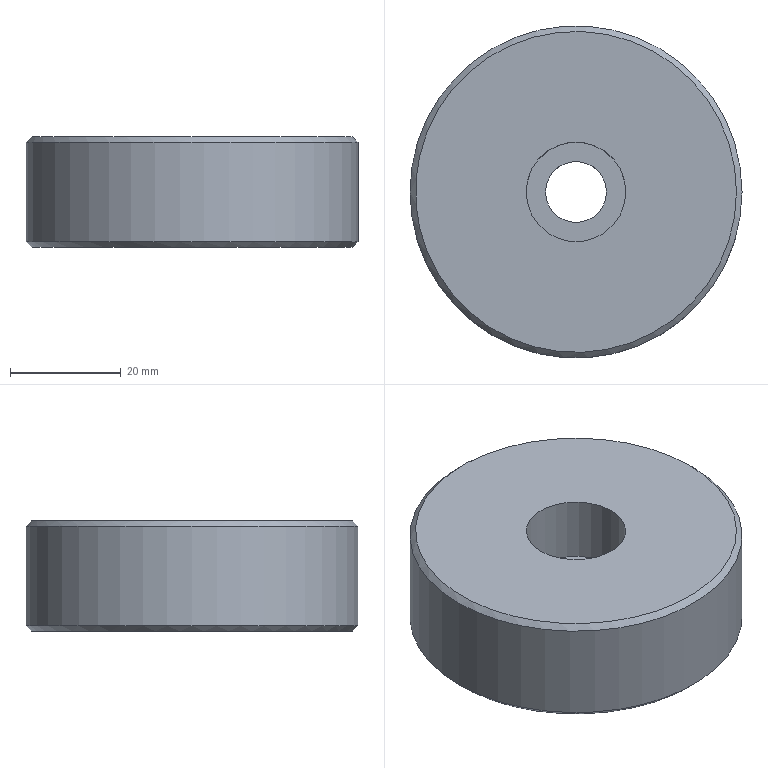Part | NX | features solid 2 | 1 solid | 8 faces | box 60 x 60 x 20 mm | volume 52548 mm3 | cylinder 3 | plane 3 | cone 2 | commonest cylinder face diameters 11 x1 18 x1 60 x1
STEP:
#1=CARTESIAN_POINT('',(975.,-425.,-19.));
#2=VERTEX_POINT('',#1);
#3=CARTESIAN_POINT('',(945.,-425.,-19.));
#4=DIRECTION('',(0.,0.,1.));
#5=DIRECTION('',(1.,0.,0.));
#6=AXIS2_PLACEMENT_3D('',#3,#4,#5);
#7=CIRCLE('',#6,30.);
#8=EDGE_CURVE('',#2,#2,#7,.T.);
#9=ORIENTED_EDGE('',*,*,#8,.T.);
#10=EDGE_LOOP('',(#9));
#11=FACE_BOUND('',#10,.T.);
#12=CARTESIAN_POINT('',(975.,-425.,-1.));
#13=VERTEX_POINT('',#12);
#14=CARTESIAN_POINT('',(945.,-425.,-1.));
#15=DIRECTION('',(0.,0.,1.));
#16=DIRECTION('',(1.,0.,0.));
#17=AXIS2_PLACEMENT_3D('',#14,#15,#16);
#18=CIRCLE('',#17,30.);
#19=EDGE_CURVE('',#13,#13,#18,.F.);
#20=ORIENTED_EDGE('',*,*,#19,.T.);
#21=EDGE_LOOP('',(#20));
#22=FACE_BOUND('',#21,.T.);
#23=CARTESIAN_POINT('',(945.,-425.,-20.));
#24=DIRECTION('',(0.,0.,1.));
#25=DIRECTION('',(1.,0.,0.));
#26=AXIS2_PLACEMENT_3D('',#23,#24,#25);
#27=CYLINDRICAL_SURFACE('',#26,30.);
#28=ADVANCED_FACE('',(#11,#22),#27,.T.);
#29=CARTESIAN_POINT('',(950.5,-425.,-20.));
#30=VERTEX_POINT('',#29);
#31=CARTESIAN_POINT('',(945.,-425.,-20.));
#32=DIRECTION('',(0.,0.,1.));
#33=DIRECTION('',(1.,0.,0.));
#34=AXIS2_PLACEMENT_3D('',#31,#32,#33);
#35=CIRCLE('',#34,5.5);
#36=EDGE_CURVE('',#30,#30,#35,.T.);
#37=ORIENTED_EDGE('',*,*,#36,.T.);
#38=EDGE_LOOP('',(#37));
#39=FACE_BOUND('',#38,.T.);
#40=CARTESIAN_POINT('',(974.,-425.,-20.));
#41=VERTEX_POINT('',#40);
#42=CARTESIAN_POINT('',(945.,-425.,-20.));
#43=DIRECTION('',(0.,0.,1.));
#44=DIRECTION('',(1.,0.,0.));
#45=AXIS2_PLACEMENT_3D('',#42,#43,#44);
#46=CIRCLE('',#45,29.);
#47=EDGE_CURVE('',#41,#41,#46,.F.);
#48=ORIENTED_EDGE('',*,*,#47,.T.);
#49=EDGE_LOOP('',(#48));
#50=FACE_BOUND('',#49,.T.);
#51=CARTESIAN_POINT('',(945.,-425.,-20.));
#52=DIRECTION('',(0.,0.,1.));
#53=DIRECTION('',(1.,0.,0.));
#54=AXIS2_PLACEMENT_3D('',#51,#52,#53);
#55=PLANE('',#54);
#56=ADVANCED_FACE('',(#39,#50),#55,.F.);
#57=CARTESIAN_POINT('',(936.,-425.,0.));
#58=VERTEX_POINT('',#57);
#59=CARTESIAN_POINT('',(945.,-425.,0.));
#60=DIRECTION('',(0.,0.,-1.));
#61=DIRECTION('',(-1.,0.,0.));
#62=AXIS2_PLACEMENT_3D('',#59,#60,#61);
#63=CIRCLE('',#62,9.);
#64=EDGE_CURVE('',#58,#58,#63,.T.);
#65=ORIENTED_EDGE('',*,*,#64,.T.);
#66=EDGE_LOOP('',(#65));
#67=FACE_BOUND('',#66,.T.);
#68=CARTESIAN_POINT('',(974.,-425.,0.));
#69=VERTEX_POINT('',#68);
#70=CARTESIAN_POINT('',(945.,-425.,0.));
#71=DIRECTION('',(0.,0.,1.));
#72=DIRECTION('',(1.,0.,0.));
#73=AXIS2_PLACEMENT_3D('',#70,#71,#72);
#74=CIRCLE('',#73,29.);
#75=EDGE_CURVE('',#69,#69,#74,.T.);
#76=ORIENTED_EDGE('',*,*,#75,.T.);
#77=EDGE_LOOP('',(#76));
#78=FACE_BOUND('',#77,.T.);
#79=CARTESIAN_POINT('',(945.,-425.,0.));
#80=DIRECTION('',(0.,0.,1.));
#81=DIRECTION('',(1.,0.,0.));
#82=AXIS2_PLACEMENT_3D('',#79,#80,#81);
#83=PLANE('',#82);
#84=ADVANCED_FACE('',(#67,#78),#83,.T.);
#85=ORIENTED_EDGE('',*,*,#47,.F.);
#86=EDGE_LOOP('',(#85));
#87=FACE_BOUND('',#86,.T.);
#88=ORIENTED_EDGE('',*,*,#8,.F.);
#89=EDGE_LOOP('',(#88));
#90=FACE_BOUND('',#89,.T.);
#91=CARTESIAN_POINT('',(945.,-425.,-19.));
#92=DIRECTION('',(0.,0.,1.));
#93=DIRECTION('',(1.,0.,0.));
#94=AXIS2_PLACEMENT_3D('',#91,#92,#93);
#95=CONICAL_SURFACE('',#94,30.,0.7854);
#96=ADVANCED_FACE('',(#87,#90),#95,.T.);
#97=ORIENTED_EDGE('',*,*,#19,.F.);
#98=EDGE_LOOP('',(#97));
#99=FACE_BOUND('',#98,.T.);
#100=ORIENTED_EDGE('',*,*,#75,.F.);
#101=EDGE_LOOP('',(#100));
#102=FACE_BOUND('',#101,.T.);
#103=CARTESIAN_POINT('',(945.,-425.,0.));
#104=DIRECTION('',(0.,0.,-1.));
#105=DIRECTION('',(-1.,0.,0.));
#106=AXIS2_PLACEMENT_3D('',#103,#104,#105);
#107=CONICAL_SURFACE('',#106,29.,0.7854);
#108=ADVANCED_FACE('',(#99,#102),#107,.T.);
#109=CARTESIAN_POINT('',(939.5,-425.,-12.));
#110=VERTEX_POINT('',#109);
#111=CARTESIAN_POINT('',(945.,-425.,-12.));
#112=DIRECTION('',(0.,0.,-1.));
#113=DIRECTION('',(-1.,0.,0.));
#114=AXIS2_PLACEMENT_3D('',#111,#112,#113);
#115=CIRCLE('',#114,5.5);
#116=EDGE_CURVE('',#110,#110,#115,.T.);
#117=ORIENTED_EDGE('',*,*,#116,.F.);
#118=EDGE_LOOP('',(#117));
#119=FACE_BOUND('',#118,.T.);
#120=ORIENTED_EDGE('',*,*,#36,.F.);
#121=EDGE_LOOP('',(#120));
#122=FACE_BOUND('',#121,.T.);
#123=CARTESIAN_POINT('',(945.,-425.,-50.));
#124=DIRECTION('',(0.,0.,-1.));
#125=DIRECTION('',(-1.,0.,0.));
#126=AXIS2_PLACEMENT_3D('',#123,#124,#125);
#127=CYLINDRICAL_SURFACE('',#126,5.5);
#128=ADVANCED_FACE('',(#119,#122),#127,.F.);
#129=ORIENTED_EDGE('',*,*,#116,.T.);
#130=EDGE_LOOP('',(#129));
#131=FACE_BOUND('',#130,.T.);
#132=CARTESIAN_POINT('',(936.,-425.,-12.));
#133=VERTEX_POINT('',#132);
#134=CARTESIAN_POINT('',(945.,-425.,-12.));
#135=DIRECTION('',(0.,0.,-1.));
#136=DIRECTION('',(-1.,0.,0.));
#137=AXIS2_PLACEMENT_3D('',#134,#135,#136);
#138=CIRCLE('',#137,9.);
#139=EDGE_CURVE('',#133,#133,#138,.T.);
#140=ORIENTED_EDGE('',*,*,#139,.F.);
#141=EDGE_LOOP('',(#140));
#142=FACE_BOUND('',#141,.T.);
#143=CARTESIAN_POINT('',(945.,-425.,-12.));
#144=DIRECTION('',(0.,0.,-1.));
#145=DIRECTION('',(-1.,0.,0.));
#146=AXIS2_PLACEMENT_3D('',#143,#144,#145);
#147=PLANE('',#146);
#148=ADVANCED_FACE('',(#131,#142),#147,.F.);
#149=ORIENTED_EDGE('',*,*,#139,.T.);
#150=EDGE_LOOP('',(#149));
#151=FACE_BOUND('',#150,.T.);
#152=ORIENTED_EDGE('',*,*,#64,.F.);
#153=EDGE_LOOP('',(#152));
#154=FACE_BOUND('',#153,.T.);
#155=CARTESIAN_POINT('',(945.,-425.,0.));
#156=DIRECTION('',(0.,0.,-1.));
#157=DIRECTION('',(-1.,0.,0.));
#158=AXIS2_PLACEMENT_3D('',#155,#156,#157);
#159=CYLINDRICAL_SURFACE('',#158,9.);
#160=ADVANCED_FACE('',(#151,#154),#159,.F.);
#161=CLOSED_SHELL('',(#28,#56,#84,#96,#108,#128,#148,#160));
#162=MANIFOLD_SOLID_BREP('',#161);
#163=(LENGTH_UNIT()NAMED_UNIT(*)SI_UNIT(.MILLI.,.METRE.));
#164=UNCERTAINTY_MEASURE_WITH_UNIT(LENGTH_MEASURE(0.00001),#163,'','');
#165=(NAMED_UNIT(*)PLANE_ANGLE_UNIT()SI_UNIT($,.RADIAN.));
#166=(NAMED_UNIT(*)SI_UNIT($,.STERADIAN.)SOLID_ANGLE_UNIT());
#167=(GEOMETRIC_REPRESENTATION_CONTEXT(3)GLOBAL_UNCERTAINTY_ASSIGNED_CONTEXT((#164))GLOBAL_UNIT_ASSIGNED_CONTEXT((#163,#165,#166))REPRESENTATION_CONTEXT('',''));
#168=ADVANCED_BREP_SHAPE_REPRESENTATION('',(#162),#167);